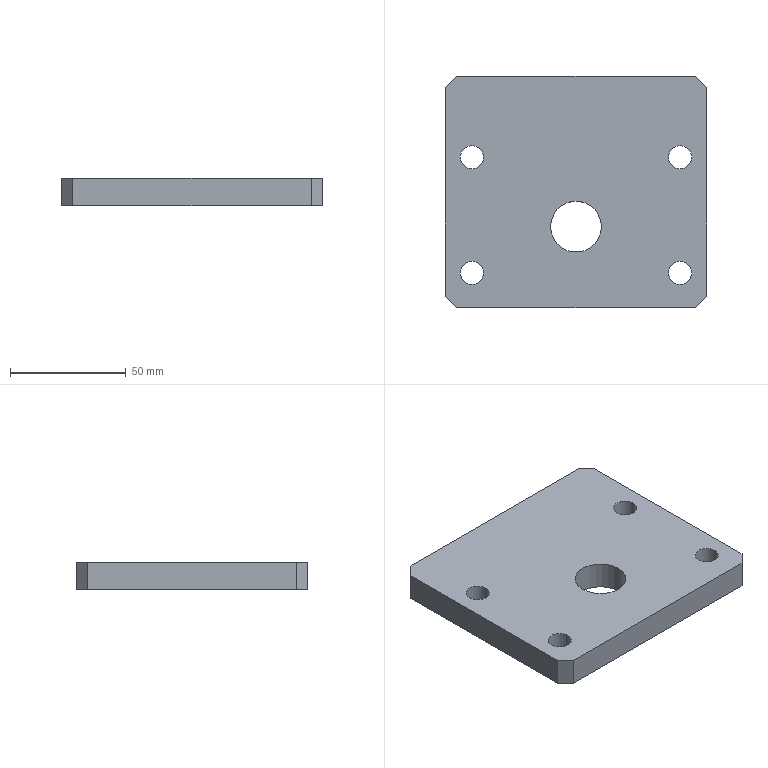Part | STEP file | J453-EBZ05-12-00-Part-1 | 1 solid | 20 faces | box 113 x 100 x 12 mm | volume 126668 mm3 | cylinder 10 | plane 10 | commonest cylinder face diameters 10 x8 22 x2